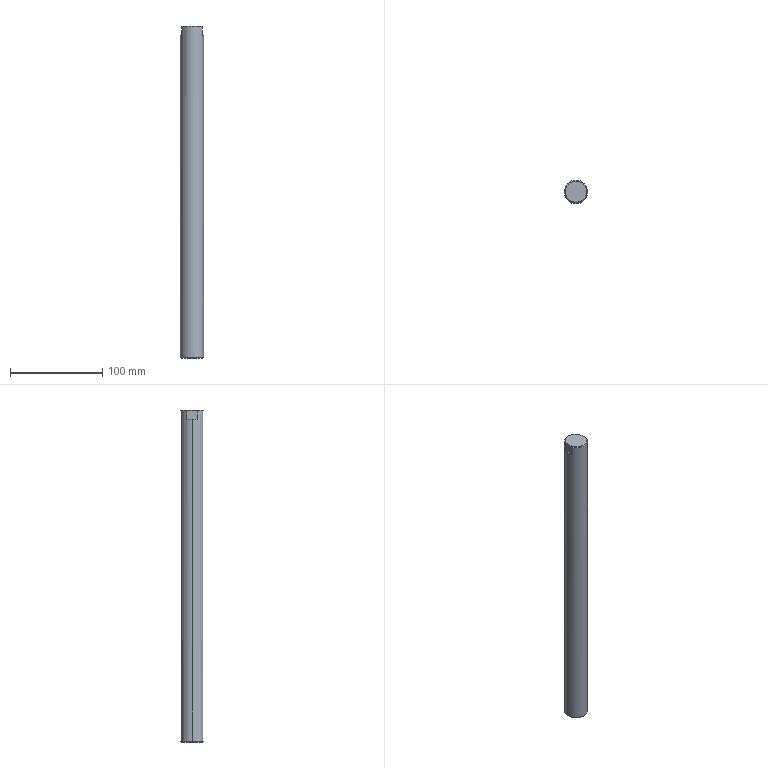Part | SolidWorks | features BaseBody 1 | 1 solid | 16 faces | box 25 x 25 x 360 mm | volume 175576 mm3 | cone 6 | plane 6 | cylinder 4 | commonest cylinder face diameters 6.8 x2 25 x2
STEP:
#1=CARTESIAN_POINT('',(3.4,0.,22.25));
#2=VERTEX_POINT('',#1);
#3=CARTESIAN_POINT('',(-3.4,0.,22.25));
#4=VERTEX_POINT('',#3);
#5=CARTESIAN_POINT('',(0.,0.,22.25));
#6=DIRECTION('',(0.,0.,-1.));
#7=DIRECTION('',(-1.,0.,0.));
#8=AXIS2_PLACEMENT_3D('',#5,#6,#7);
#9=CIRCLE('',#8,3.4);
#10=EDGE_CURVE('',#2,#4,#9,.T.);
#11=ORIENTED_EDGE('',*,*,#10,.F.);
#12=CARTESIAN_POINT('',(3.4,0.,0.));
#13=VERTEX_POINT('',#12);
#14=CARTESIAN_POINT('',(3.4,0.,0.));
#15=DIRECTION('',(0.,0.,-1.));
#16=VECTOR('',#15,1000.);
#17=LINE('',#14,#16);
#18=EDGE_CURVE('',#2,#13,#17,.T.);
#19=ORIENTED_EDGE('',*,*,#18,.T.);
#20=CARTESIAN_POINT('',(-3.4,0.,0.));
#21=VERTEX_POINT('',#20);
#22=CARTESIAN_POINT('',(0.,0.,0.));
#23=DIRECTION('',(0.,0.,-1.));
#24=DIRECTION('',(-1.,0.,0.));
#25=AXIS2_PLACEMENT_3D('',#22,#23,#24);
#26=CIRCLE('',#25,3.4);
#27=EDGE_CURVE('',#13,#21,#26,.T.);
#28=ORIENTED_EDGE('',*,*,#27,.T.);
#29=CARTESIAN_POINT('',(-3.4,0.,0.));
#30=DIRECTION('',(0.,0.,-1.));
#31=VECTOR('',#30,1000.);
#32=LINE('',#29,#31);
#33=EDGE_CURVE('',#4,#21,#32,.T.);
#34=ORIENTED_EDGE('',*,*,#33,.F.);
#35=EDGE_LOOP('',(#11,#19,#28,#34));
#36=FACE_OUTER_BOUND('',#35,.T.);
#37=CARTESIAN_POINT('',(0.,0.,0.));
#38=DIRECTION('',(0.,0.,-1.));
#39=DIRECTION('',(-1.,0.,0.));
#40=AXIS2_PLACEMENT_3D('',#37,#38,#39);
#41=CYLINDRICAL_SURFACE('',#40,3.4);
#42=ADVANCED_FACE('',(#36),#41,.F.);
#43=CARTESIAN_POINT('',(0.,0.,24.293));
#44=VERTEX_POINT('',#43);
#45=CARTESIAN_POINT('',(-3.4,0.,22.25));
#46=DIRECTION('',(-0.8572,0.,-0.515));
#47=VECTOR('',#46,1000.);
#48=LINE('',#45,#47);
#49=EDGE_CURVE('',#44,#4,#48,.T.);
#50=ORIENTED_EDGE('',*,*,#49,.F.);
#51=CARTESIAN_POINT('',(3.4,0.,22.25));
#52=DIRECTION('',(0.8572,0.,-0.515));
#53=VECTOR('',#52,1000.);
#54=LINE('',#51,#53);
#55=EDGE_CURVE('',#44,#2,#54,.T.);
#56=ORIENTED_EDGE('',*,*,#55,.T.);
#57=ORIENTED_EDGE('',*,*,#10,.T.);
#58=EDGE_LOOP('',(#50,#56,#57));
#59=FACE_OUTER_BOUND('',#58,.T.);
#60=CARTESIAN_POINT('',(0.,0.,22.25));
#61=DIRECTION('',(0.,0.,-1.));
#62=DIRECTION('',(-1.,0.,0.));
#63=AXIS2_PLACEMENT_3D('',#60,#61,#62);
#64=CONICAL_SURFACE('',#63,3.4,1.03);
#65=ADVANCED_FACE('',(#59),#64,.F.);
#66=CARTESIAN_POINT('',(-11.5,0.,0.));
#67=VERTEX_POINT('',#66);
#68=CARTESIAN_POINT('',(11.5,0.,0.));
#69=VERTEX_POINT('',#68);
#70=CARTESIAN_POINT('',(0.,0.,0.));
#71=DIRECTION('',(0.,0.,-1.));
#72=DIRECTION('',(1.,0.,0.));
#73=AXIS2_PLACEMENT_3D('',#70,#71,#72);
#74=CIRCLE('',#73,11.5);
#75=EDGE_CURVE('',#67,#69,#74,.T.);
#76=ORIENTED_EDGE('',*,*,#75,.F.);
#77=CARTESIAN_POINT('',(-12.5,0.,1.));
#78=VERTEX_POINT('',#77);
#79=CARTESIAN_POINT('',(-12.5,0.,1.));
#80=DIRECTION('',(-0.7071,0.,0.7071));
#81=VECTOR('',#80,1000.);
#82=LINE('',#79,#81);
#83=EDGE_CURVE('',#67,#78,#82,.T.);
#84=ORIENTED_EDGE('',*,*,#83,.T.);
#85=CARTESIAN_POINT('',(12.5,0.,1.));
#86=VERTEX_POINT('',#85);
#87=CARTESIAN_POINT('',(0.,0.,1.));
#88=DIRECTION('',(0.,0.,1.));
#89=DIRECTION('',(1.,0.,0.));
#90=AXIS2_PLACEMENT_3D('',#87,#88,#89);
#91=CIRCLE('',#90,12.5);
#92=EDGE_CURVE('',#86,#78,#91,.T.);
#93=ORIENTED_EDGE('',*,*,#92,.F.);
#94=CARTESIAN_POINT('',(12.5,0.,1.));
#95=DIRECTION('',(0.7071,0.,0.7071));
#96=VECTOR('',#95,1000.);
#97=LINE('',#94,#96);
#98=EDGE_CURVE('',#69,#86,#97,.T.);
#99=ORIENTED_EDGE('',*,*,#98,.F.);
#100=EDGE_LOOP('',(#76,#84,#93,#99));
#101=FACE_OUTER_BOUND('',#100,.T.);
#102=CARTESIAN_POINT('',(0.,0.,1.));
#103=DIRECTION('',(0.,0.,1.));
#104=DIRECTION('',(1.,0.,0.));
#105=AXIS2_PLACEMENT_3D('',#102,#103,#104);
#106=CONICAL_SURFACE('',#105,12.5,0.7854);
#107=ADVANCED_FACE('',(#101),#106,.T.);
#108=CARTESIAN_POINT('',(12.5,0.,350.));
#109=VERTEX_POINT('',#108);
#110=CARTESIAN_POINT('',(11.,5.937,350.));
#111=VERTEX_POINT('',#110);
#112=CARTESIAN_POINT('',(0.,0.,350.));
#113=DIRECTION('',(0.,0.,1.));
#114=DIRECTION('',(1.,0.,0.));
#115=AXIS2_PLACEMENT_3D('',#112,#113,#114);
#116=CIRCLE('',#115,12.5);
#117=EDGE_CURVE('',#109,#111,#116,.T.);
#118=ORIENTED_EDGE('',*,*,#117,.F.);
#119=CARTESIAN_POINT('',(12.5,0.,360.));
#120=DIRECTION('',(0.,0.,-1.));
#121=VECTOR('',#120,1000.);
#122=LINE('',#119,#121);
#123=EDGE_CURVE('',#109,#86,#122,.T.);
#124=ORIENTED_EDGE('',*,*,#123,.T.);
#125=ORIENTED_EDGE('',*,*,#92,.T.);
#126=CARTESIAN_POINT('',(-12.5,0.,350.));
#127=VERTEX_POINT('',#126);
#128=CARTESIAN_POINT('',(-12.5,0.,360.));
#129=DIRECTION('',(0.,0.,-1.));
#130=VECTOR('',#129,1000.);
#131=LINE('',#128,#130);
#132=EDGE_CURVE('',#127,#78,#131,.T.);
#133=ORIENTED_EDGE('',*,*,#132,.F.);
#134=CARTESIAN_POINT('',(-11.,5.937,350.));
#135=VERTEX_POINT('',#134);
#136=CARTESIAN_POINT('',(0.,0.,350.));
#137=DIRECTION('',(0.,0.,1.));
#138=DIRECTION('',(1.,0.,0.));
#139=AXIS2_PLACEMENT_3D('',#136,#137,#138);
#140=CIRCLE('',#139,12.5);
#141=EDGE_CURVE('',#135,#127,#140,.T.);
#142=ORIENTED_EDGE('',*,*,#141,.F.);
#143=CARTESIAN_POINT('',(-11.,5.937,359.));
#144=VERTEX_POINT('',#143);
#145=CARTESIAN_POINT('',(-11.,5.937,360.));
#146=DIRECTION('',(0.,0.,1.));
#147=VECTOR('',#146,1000.);
#148=LINE('',#145,#147);
#149=EDGE_CURVE('',#135,#144,#148,.T.);
#150=ORIENTED_EDGE('',*,*,#149,.T.);
#151=CARTESIAN_POINT('',(11.,5.937,359.));
#152=VERTEX_POINT('',#151);
#153=CARTESIAN_POINT('',(0.,0.,359.));
#154=DIRECTION('',(0.,0.,-1.));
#155=DIRECTION('',(1.,0.,0.));
#156=AXIS2_PLACEMENT_3D('',#153,#154,#155);
#157=CIRCLE('',#156,12.5);
#158=EDGE_CURVE('',#144,#152,#157,.T.);
#159=ORIENTED_EDGE('',*,*,#158,.T.);
#160=CARTESIAN_POINT('',(11.,5.937,360.));
#161=DIRECTION('',(0.,0.,-1.));
#162=VECTOR('',#161,1000.);
#163=LINE('',#160,#162);
#164=EDGE_CURVE('',#152,#111,#163,.T.);
#165=ORIENTED_EDGE('',*,*,#164,.T.);
#166=EDGE_LOOP('',(#118,#124,#125,#133,#142,#150,#159,#165));
#167=FACE_OUTER_BOUND('',#166,.T.);
#168=CARTESIAN_POINT('',(0.,0.,360.));
#169=DIRECTION('',(0.,0.,-1.));
#170=DIRECTION('',(-1.,0.,0.));
#171=AXIS2_PLACEMENT_3D('',#168,#169,#170);
#172=CYLINDRICAL_SURFACE('',#171,12.5);
#173=ADVANCED_FACE('',(#167),#172,.T.);
#174=CARTESIAN_POINT('',(11.,3.354,360.));
#175=VERTEX_POINT('',#174);
#176=CARTESIAN_POINT('',(11.,5.937,359.));
#177=CARTESIAN_POINT('',(11.,5.522,359.197));
#178=CARTESIAN_POINT('',(11.,5.1,359.382));
#179=CARTESIAN_POINT('',(11.,4.24,359.718));
#180=CARTESIAN_POINT('',(11.,3.8,359.87));
#181=CARTESIAN_POINT('',(11.,3.354,360.));
#182=B_SPLINE_CURVE_WITH_KNOTS('',3,(#176,#177,#178,#179,#180,#181),.UNSPECIFIED.,.F.,.F.,(4,2,4),(0.01313,0.01451,0.0159),.UNSPECIFIED.);
#183=EDGE_CURVE('',#152,#175,#182,.T.);
#184=ORIENTED_EDGE('',*,*,#183,.F.);
#185=ORIENTED_EDGE('',*,*,#158,.F.);
#186=CARTESIAN_POINT('',(-11.,3.354,360.));
#187=VERTEX_POINT('',#186);
#188=CARTESIAN_POINT('',(-11.,3.354,360.));
#189=CARTESIAN_POINT('',(-11.,3.795,359.871));
#190=CARTESIAN_POINT('',(-11.,4.231,359.721));
#191=CARTESIAN_POINT('',(-11.,5.095,359.384));
#192=CARTESIAN_POINT('',(-11.,5.521,359.198));
#193=CARTESIAN_POINT('',(-11.,5.937,359.));
#194=B_SPLINE_CURVE_WITH_KNOTS('',3,(#188,#189,#190,#191,#192,#193),.UNSPECIFIED.,.F.,.F.,(4,2,4),(0.02667,0.02805,0.02943),.UNSPECIFIED.);
#195=EDGE_CURVE('',#187,#144,#194,.T.);
#196=ORIENTED_EDGE('',*,*,#195,.F.);
#197=CARTESIAN_POINT('',(0.,0.,360.));
#198=DIRECTION('',(0.,0.,1.));
#199=DIRECTION('',(1.,0.,0.));
#200=AXIS2_PLACEMENT_3D('',#197,#198,#199);
#201=CIRCLE('',#200,11.5);
#202=EDGE_CURVE('',#175,#187,#201,.T.);
#203=ORIENTED_EDGE('',*,*,#202,.F.);
#204=EDGE_LOOP('',(#184,#185,#196,#203));
#205=FACE_OUTER_BOUND('',#204,.T.);
#206=CARTESIAN_POINT('',(0.,0.,360.));
#207=DIRECTION('',(0.,0.,-1.));
#208=DIRECTION('',(-1.,0.,0.));
#209=AXIS2_PLACEMENT_3D('',#206,#207,#208);
#210=CONICAL_SURFACE('',#209,11.5,0.7854);
#211=ADVANCED_FACE('',(#205),#210,.T.);
#212=ORIENTED_EDGE('',*,*,#123,.F.);
#213=CARTESIAN_POINT('',(11.,-5.937,350.));
#214=VERTEX_POINT('',#213);
#215=CARTESIAN_POINT('',(0.,0.,350.));
#216=DIRECTION('',(0.,0.,1.));
#217=DIRECTION('',(1.,0.,0.));
#218=AXIS2_PLACEMENT_3D('',#215,#216,#217);
#219=CIRCLE('',#218,12.5);
#220=EDGE_CURVE('',#214,#109,#219,.T.);
#221=ORIENTED_EDGE('',*,*,#220,.F.);
#222=CARTESIAN_POINT('',(11.,-5.937,359.));
#223=VERTEX_POINT('',#222);
#224=CARTESIAN_POINT('',(11.,-5.937,360.));
#225=DIRECTION('',(0.,0.,1.));
#226=VECTOR('',#225,1000.);
#227=LINE('',#224,#226);
#228=EDGE_CURVE('',#214,#223,#227,.T.);
#229=ORIENTED_EDGE('',*,*,#228,.T.);
#230=CARTESIAN_POINT('',(-11.,-5.937,359.));
#231=VERTEX_POINT('',#230);
#232=CARTESIAN_POINT('',(0.,0.,359.));
#233=DIRECTION('',(0.,0.,-1.));
#234=DIRECTION('',(1.,0.,0.));
#235=AXIS2_PLACEMENT_3D('',#232,#233,#234);
#236=CIRCLE('',#235,12.5);
#237=EDGE_CURVE('',#223,#231,#236,.T.);
#238=ORIENTED_EDGE('',*,*,#237,.T.);
#239=CARTESIAN_POINT('',(-11.,-5.937,350.));
#240=VERTEX_POINT('',#239);
#241=CARTESIAN_POINT('',(-11.,-5.937,360.));
#242=DIRECTION('',(0.,0.,-1.));
#243=VECTOR('',#242,1000.);
#244=LINE('',#241,#243);
#245=EDGE_CURVE('',#231,#240,#244,.T.);
#246=ORIENTED_EDGE('',*,*,#245,.T.);
#247=CARTESIAN_POINT('',(0.,0.,350.));
#248=DIRECTION('',(0.,0.,1.));
#249=DIRECTION('',(1.,0.,0.));
#250=AXIS2_PLACEMENT_3D('',#247,#248,#249);
#251=CIRCLE('',#250,12.5);
#252=EDGE_CURVE('',#127,#240,#251,.T.);
#253=ORIENTED_EDGE('',*,*,#252,.F.);
#254=ORIENTED_EDGE('',*,*,#132,.T.);
#255=CARTESIAN_POINT('',(0.,0.,1.));
#256=DIRECTION('',(0.,0.,1.));
#257=DIRECTION('',(1.,0.,0.));
#258=AXIS2_PLACEMENT_3D('',#255,#256,#257);
#259=CIRCLE('',#258,12.5);
#260=EDGE_CURVE('',#78,#86,#259,.T.);
#261=ORIENTED_EDGE('',*,*,#260,.T.);
#262=EDGE_LOOP('',(#212,#221,#229,#238,#246,#253,#254,#261));
#263=FACE_OUTER_BOUND('',#262,.T.);
#264=CARTESIAN_POINT('',(0.,0.,360.));
#265=DIRECTION('',(0.,0.,-1.));
#266=DIRECTION('',(-1.,0.,0.));
#267=AXIS2_PLACEMENT_3D('',#264,#265,#266);
#268=CYLINDRICAL_SURFACE('',#267,12.5);
#269=ADVANCED_FACE('',(#263),#268,.T.);
#270=CARTESIAN_POINT('',(11.,-3.354,360.));
#271=VERTEX_POINT('',#270);
#272=CARTESIAN_POINT('',(11.,6.621,360.));
#273=DIRECTION('',(0.,-1.,0.));
#274=VECTOR('',#273,1000.);
#275=LINE('',#272,#274);
#276=EDGE_CURVE('',#175,#271,#275,.T.);
#277=ORIENTED_EDGE('',*,*,#276,.F.);
#278=ORIENTED_EDGE('',*,*,#202,.T.);
#279=CARTESIAN_POINT('',(-11.,-3.354,360.));
#280=VERTEX_POINT('',#279);
#281=CARTESIAN_POINT('',(-11.,6.621,360.));
#282=DIRECTION('',(0.,1.,0.));
#283=VECTOR('',#282,1000.);
#284=LINE('',#281,#283);
#285=EDGE_CURVE('',#280,#187,#284,.T.);
#286=ORIENTED_EDGE('',*,*,#285,.F.);
#287=CARTESIAN_POINT('',(0.,0.,360.));
#288=DIRECTION('',(0.,0.,1.));
#289=DIRECTION('',(1.,0.,0.));
#290=AXIS2_PLACEMENT_3D('',#287,#288,#289);
#291=CIRCLE('',#290,11.5);
#292=EDGE_CURVE('',#280,#271,#291,.T.);
#293=ORIENTED_EDGE('',*,*,#292,.T.);
#294=EDGE_LOOP('',(#277,#278,#286,#293));
#295=FACE_OUTER_BOUND('',#294,.T.);
#296=CARTESIAN_POINT('',(0.,0.,360.));
#297=DIRECTION('',(0.,0.,1.));
#298=DIRECTION('',(1.,0.,0.));
#299=AXIS2_PLACEMENT_3D('',#296,#297,#298);
#300=PLANE('',#299);
#301=ADVANCED_FACE('',(#295),#300,.T.);
#302=CARTESIAN_POINT('',(0.,0.,0.));
#303=DIRECTION('',(0.,0.,-1.));
#304=DIRECTION('',(-1.,0.,0.));
#305=AXIS2_PLACEMENT_3D('',#302,#303,#304);
#306=CIRCLE('',#305,3.4);
#307=EDGE_CURVE('',#21,#13,#306,.T.);
#308=ORIENTED_EDGE('',*,*,#307,.F.);
#309=ORIENTED_EDGE('',*,*,#27,.F.);
#310=EDGE_LOOP('',(#308,#309));
#311=FACE_BOUND('',#310,.T.);
#312=CARTESIAN_POINT('',(0.,0.,0.));
#313=DIRECTION('',(0.,0.,-1.));
#314=DIRECTION('',(1.,0.,0.));
#315=AXIS2_PLACEMENT_3D('',#312,#313,#314);
#316=CIRCLE('',#315,11.5);
#317=EDGE_CURVE('',#69,#67,#316,.T.);
#318=ORIENTED_EDGE('',*,*,#317,.T.);
#319=ORIENTED_EDGE('',*,*,#75,.T.);
#320=EDGE_LOOP('',(#318,#319));
#321=FACE_OUTER_BOUND('',#320,.T.);
#322=CARTESIAN_POINT('',(0.,0.,0.));
#323=DIRECTION('',(0.,0.,1.));
#324=DIRECTION('',(1.,0.,0.));
#325=AXIS2_PLACEMENT_3D('',#322,#323,#324);
#326=PLANE('',#325);
#327=ADVANCED_FACE('',(#311,#321),#326,.F.);
#328=ORIENTED_EDGE('',*,*,#83,.F.);
#329=ORIENTED_EDGE('',*,*,#317,.F.);
#330=ORIENTED_EDGE('',*,*,#98,.T.);
#331=ORIENTED_EDGE('',*,*,#260,.F.);
#332=EDGE_LOOP('',(#328,#329,#330,#331));
#333=FACE_OUTER_BOUND('',#332,.T.);
#334=CARTESIAN_POINT('',(0.,0.,1.));
#335=DIRECTION('',(0.,0.,1.));
#336=DIRECTION('',(1.,0.,0.));
#337=AXIS2_PLACEMENT_3D('',#334,#335,#336);
#338=CONICAL_SURFACE('',#337,12.5,0.7854);
#339=ADVANCED_FACE('',(#333),#338,.T.);
#340=CARTESIAN_POINT('',(11.,-3.354,360.));
#341=CARTESIAN_POINT('',(11.,-3.797,359.871));
#342=CARTESIAN_POINT('',(11.,-4.237,359.719));
#343=CARTESIAN_POINT('',(11.,-5.1,359.382));
#344=CARTESIAN_POINT('',(11.,-5.522,359.197));
#345=CARTESIAN_POINT('',(11.,-5.937,359.));
#346=B_SPLINE_CURVE_WITH_KNOTS('',3,(#340,#341,#342,#343,#344,#345),.UNSPECIFIED.,.F.,.F.,(4,2,4),(0.02269,0.02408,0.02546),.UNSPECIFIED.);
#347=EDGE_CURVE('',#271,#223,#346,.T.);
#348=ORIENTED_EDGE('',*,*,#347,.F.);
#349=ORIENTED_EDGE('',*,*,#292,.F.);
#350=CARTESIAN_POINT('',(-11.,-5.937,359.));
#351=CARTESIAN_POINT('',(-11.,-5.522,359.197));
#352=CARTESIAN_POINT('',(-11.,-5.1,359.382));
#353=CARTESIAN_POINT('',(-11.,-4.236,359.719));
#354=CARTESIAN_POINT('',(-11.,-3.796,359.871));
#355=CARTESIAN_POINT('',(-11.,-3.354,360.));
#356=B_SPLINE_CURVE_WITH_KNOTS('',3,(#350,#351,#352,#353,#354,#355),.UNSPECIFIED.,.F.,.F.,(4,2,4),(0.01711,0.01849,0.01987),.UNSPECIFIED.);
#357=EDGE_CURVE('',#231,#280,#356,.T.);
#358=ORIENTED_EDGE('',*,*,#357,.F.);
#359=ORIENTED_EDGE('',*,*,#237,.F.);
#360=EDGE_LOOP('',(#348,#349,#358,#359));
#361=FACE_OUTER_BOUND('',#360,.T.);
#362=CARTESIAN_POINT('',(0.,0.,360.));
#363=DIRECTION('',(0.,0.,-1.));
#364=DIRECTION('',(-1.,0.,0.));
#365=AXIS2_PLACEMENT_3D('',#362,#363,#364);
#366=CONICAL_SURFACE('',#365,11.5,0.7854);
#367=ADVANCED_FACE('',(#361),#366,.T.);
#368=ORIENTED_EDGE('',*,*,#55,.F.);
#369=ORIENTED_EDGE('',*,*,#49,.T.);
#370=CARTESIAN_POINT('',(0.,0.,22.25));
#371=DIRECTION('',(0.,0.,-1.));
#372=DIRECTION('',(-1.,0.,0.));
#373=AXIS2_PLACEMENT_3D('',#370,#371,#372);
#374=CIRCLE('',#373,3.4);
#375=EDGE_CURVE('',#4,#2,#374,.T.);
#376=ORIENTED_EDGE('',*,*,#375,.T.);
#377=EDGE_LOOP('',(#368,#369,#376));
#378=FACE_OUTER_BOUND('',#377,.T.);
#379=CARTESIAN_POINT('',(0.,0.,22.25));
#380=DIRECTION('',(0.,0.,-1.));
#381=DIRECTION('',(-1.,0.,0.));
#382=AXIS2_PLACEMENT_3D('',#379,#380,#381);
#383=CONICAL_SURFACE('',#382,3.4,1.03);
#384=ADVANCED_FACE('',(#378),#383,.F.);
#385=ORIENTED_EDGE('',*,*,#18,.F.);
#386=ORIENTED_EDGE('',*,*,#375,.F.);
#387=ORIENTED_EDGE('',*,*,#33,.T.);
#388=ORIENTED_EDGE('',*,*,#307,.T.);
#389=EDGE_LOOP('',(#385,#386,#387,#388));
#390=FACE_OUTER_BOUND('',#389,.T.);
#391=CARTESIAN_POINT('',(0.,0.,0.));
#392=DIRECTION('',(0.,0.,-1.));
#393=DIRECTION('',(-1.,0.,0.));
#394=AXIS2_PLACEMENT_3D('',#391,#392,#393);
#395=CYLINDRICAL_SURFACE('',#394,3.4);
#396=ADVANCED_FACE('',(#390),#395,.F.);
#397=ORIENTED_EDGE('',*,*,#141,.T.);
#398=ORIENTED_EDGE('',*,*,#252,.T.);
#399=CARTESIAN_POINT('',(-11.,6.621,350.));
#400=DIRECTION('',(0.,1.,0.));
#401=VECTOR('',#400,1000.);
#402=LINE('',#399,#401);
#403=EDGE_CURVE('',#240,#135,#402,.T.);
#404=ORIENTED_EDGE('',*,*,#403,.T.);
#405=EDGE_LOOP('',(#397,#398,#404));
#406=FACE_OUTER_BOUND('',#405,.T.);
#407=CARTESIAN_POINT('',(0.,0.,350.));
#408=DIRECTION('',(0.,0.,1.));
#409=DIRECTION('',(1.,0.,0.));
#410=AXIS2_PLACEMENT_3D('',#407,#408,#409);
#411=PLANE('',#410);
#412=ADVANCED_FACE('',(#406),#411,.T.);
#413=ORIENTED_EDGE('',*,*,#357,.T.);
#414=ORIENTED_EDGE('',*,*,#285,.T.);
#415=ORIENTED_EDGE('',*,*,#195,.T.);
#416=ORIENTED_EDGE('',*,*,#149,.F.);
#417=ORIENTED_EDGE('',*,*,#403,.F.);
#418=ORIENTED_EDGE('',*,*,#245,.F.);
#419=EDGE_LOOP('',(#413,#414,#415,#416,#417,#418));
#420=FACE_OUTER_BOUND('',#419,.T.);
#421=CARTESIAN_POINT('',(-11.,6.621,350.));
#422=DIRECTION('',(1.,0.,0.));
#423=DIRECTION('',(0.,1.,0.));
#424=AXIS2_PLACEMENT_3D('',#421,#422,#423);
#425=PLANE('',#424);
#426=ADVANCED_FACE('',(#420),#425,.F.);
#427=ORIENTED_EDGE('',*,*,#220,.T.);
#428=ORIENTED_EDGE('',*,*,#117,.T.);
#429=CARTESIAN_POINT('',(11.,6.621,350.));
#430=DIRECTION('',(0.,-1.,0.));
#431=VECTOR('',#430,1000.);
#432=LINE('',#429,#431);
#433=EDGE_CURVE('',#111,#214,#432,.T.);
#434=ORIENTED_EDGE('',*,*,#433,.T.);
#435=EDGE_LOOP('',(#427,#428,#434));
#436=FACE_OUTER_BOUND('',#435,.T.);
#437=CARTESIAN_POINT('',(0.,0.,350.));
#438=DIRECTION('',(0.,0.,1.));
#439=DIRECTION('',(1.,0.,0.));
#440=AXIS2_PLACEMENT_3D('',#437,#438,#439);
#441=PLANE('',#440);
#442=ADVANCED_FACE('',(#436),#441,.T.);
#443=ORIENTED_EDGE('',*,*,#183,.T.);
#444=ORIENTED_EDGE('',*,*,#276,.T.);
#445=ORIENTED_EDGE('',*,*,#347,.T.);
#446=ORIENTED_EDGE('',*,*,#228,.F.);
#447=ORIENTED_EDGE('',*,*,#433,.F.);
#448=ORIENTED_EDGE('',*,*,#164,.F.);
#449=EDGE_LOOP('',(#443,#444,#445,#446,#447,#448));
#450=FACE_OUTER_BOUND('',#449,.T.);
#451=CARTESIAN_POINT('',(11.,6.621,350.));
#452=DIRECTION('',(-1.,0.,0.));
#453=DIRECTION('',(0.,-1.,0.));
#454=AXIS2_PLACEMENT_3D('',#451,#452,#453);
#455=PLANE('',#454);
#456=ADVANCED_FACE('',(#450),#455,.F.);
#457=CLOSED_SHELL('',(#42,#65,#107,#173,#211,#269,#301,#327,#339,#367,#384,#396,#412,#426,#442,#456));
#458=MANIFOLD_SOLID_BREP('',#457);
#459=CARTESIAN_POINT('',(0.,0.,0.));
#460=DIRECTION('',(0.,0.,1.));
#461=DIRECTION('',(1.,0.,0.));
#462=AXIS2_PLACEMENT_3D('',#459,#460,#461);
#463=(LENGTH_UNIT()NAMED_UNIT(*)SI_UNIT(.MILLI.,.METRE.));
#464=UNCERTAINTY_MEASURE_WITH_UNIT(LENGTH_MEASURE(0.00001),#463,'','');
#465=(NAMED_UNIT(*)PLANE_ANGLE_UNIT()SI_UNIT($,.RADIAN.));
#466=(NAMED_UNIT(*)SI_UNIT($,.STERADIAN.)SOLID_ANGLE_UNIT());
#467=(GEOMETRIC_REPRESENTATION_CONTEXT(3)GLOBAL_UNCERTAINTY_ASSIGNED_CONTEXT((#464))GLOBAL_UNIT_ASSIGNED_CONTEXT((#463,#465,#466))REPRESENTATION_CONTEXT('',''));
#468=ADVANCED_BREP_SHAPE_REPRESENTATION('',(#458,#462),#467);